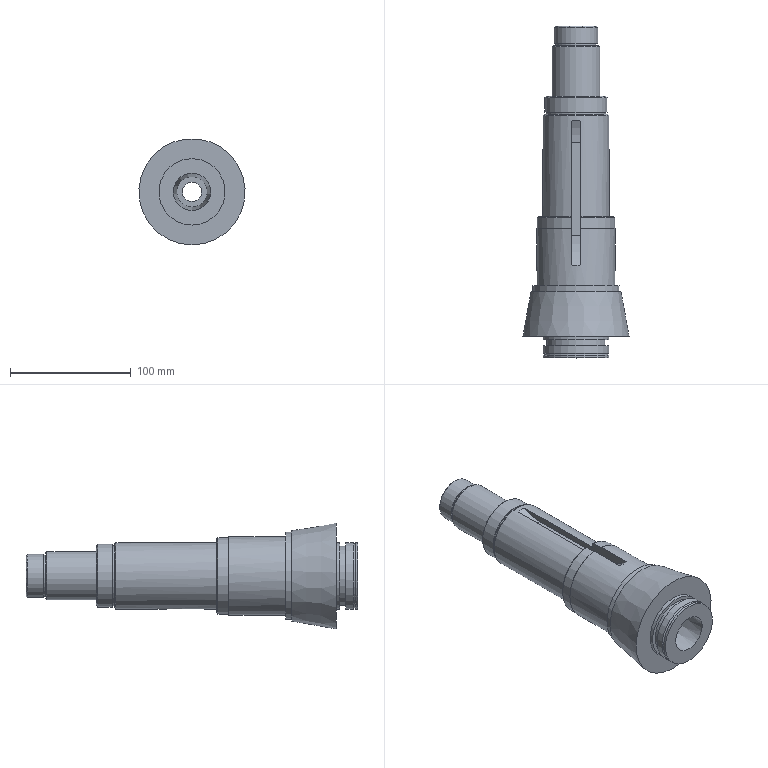Part | NX | features DATUM_CSYS 4, SKETCH 3, EXTRUDE 2, SYMBOLIC_THREAD 2, CHAMFER 1, DATUM_PLANE 1, SWP104 1 | 1 solid | 49 faces | box 88 x 275 x 88 mm | volume 636397 mm3 | plane 22 | cylinder 19 | cone 7 | torus 1 | commonest cylinder face diameters 55 x4 8 x2 70 x2 16 x1 28 x1 34 x1
STEP:
#1=CARTESIAN_POINT('',(0.,0.,-15.5));
#2=VERTEX_POINT('',#1);
#3=CARTESIAN_POINT('',(0.,0.,0.));
#4=DIRECTION('',(0.,-1.,0.));
#5=DIRECTION('',(0.,0.,-1.));
#6=AXIS2_PLACEMENT_3D('',#3,#4,#5);
#7=CIRCLE('',#6,15.5);
#8=EDGE_CURVE('',#2,#2,#7,.F.);
#9=ORIENTED_EDGE('',*,*,#8,.T.);
#10=EDGE_LOOP('',(#9));
#11=FACE_BOUND('',#10,.T.);
#12=CARTESIAN_POINT('',(0.,0.,-27.5));
#13=VERTEX_POINT('',#12);
#14=CARTESIAN_POINT('',(0.,0.,0.));
#15=DIRECTION('',(0.,-1.,0.));
#16=DIRECTION('',(0.,0.,-1.));
#17=AXIS2_PLACEMENT_3D('',#14,#15,#16);
#18=CIRCLE('',#17,27.5);
#19=EDGE_CURVE('',#13,#13,#18,.F.);
#20=ORIENTED_EDGE('',*,*,#19,.F.);
#21=EDGE_LOOP('',(#20));
#22=FACE_BOUND('',#21,.T.);
#23=CARTESIAN_POINT('',(0.,0.,27.5));
#24=DIRECTION('',(0.,1.,0.));
#25=DIRECTION('',(0.,0.,1.));
#26=AXIS2_PLACEMENT_3D('',#23,#24,#25);
#27=PLANE('',#26);
#28=ADVANCED_FACE('',(#11,#22),#27,.F.);
#29=CARTESIAN_POINT('',(0.,92.,-12.625));
#30=VERTEX_POINT('',#29);
#31=CARTESIAN_POINT('',(0.,92.,0.));
#32=DIRECTION('',(0.,-1.,0.));
#33=DIRECTION('',(0.,0.,-1.));
#34=AXIS2_PLACEMENT_3D('',#31,#32,#33);
#35=CIRCLE('',#34,12.625);
#36=EDGE_CURVE('',#30,#30,#35,.F.);
#37=ORIENTED_EDGE('',*,*,#36,.T.);
#38=EDGE_LOOP('',(#37));
#39=FACE_BOUND('',#38,.T.);
#40=ORIENTED_EDGE('',*,*,#8,.F.);
#41=EDGE_LOOP('',(#40));
#42=FACE_BOUND('',#41,.T.);
#43=CARTESIAN_POINT('',(0.,0.,0.));
#44=DIRECTION('',(0.,-1.,0.));
#45=DIRECTION('',(0.,0.,-1.));
#46=AXIS2_PLACEMENT_3D('',#43,#44,#45);
#47=CONICAL_SURFACE('',#46,15.5,0.03124);
#48=ADVANCED_FACE('',(#39,#42),#47,.F.);
#49=CARTESIAN_POINT('',(0.,92.,-14.));
#50=VERTEX_POINT('',#49);
#51=CARTESIAN_POINT('',(0.,92.,0.));
#52=DIRECTION('',(0.,-1.,0.));
#53=DIRECTION('',(0.,0.,-1.));
#54=AXIS2_PLACEMENT_3D('',#51,#52,#53);
#55=CIRCLE('',#54,14.);
#56=EDGE_CURVE('',#50,#50,#55,.F.);
#57=ORIENTED_EDGE('',*,*,#56,.T.);
#58=EDGE_LOOP('',(#57));
#59=FACE_BOUND('',#58,.T.);
#60=ORIENTED_EDGE('',*,*,#36,.F.);
#61=EDGE_LOOP('',(#60));
#62=FACE_BOUND('',#61,.T.);
#63=CARTESIAN_POINT('',(0.,92.,12.625));
#64=DIRECTION('',(0.,-1.,0.));
#65=DIRECTION('',(0.,0.,-1.));
#66=AXIS2_PLACEMENT_3D('',#63,#64,#65);
#67=PLANE('',#66);
#68=ADVANCED_FACE('',(#59,#62),#67,.F.);
#69=CARTESIAN_POINT('',(0.,107.,-14.));
#70=VERTEX_POINT('',#69);
#71=CARTESIAN_POINT('',(0.,107.,0.));
#72=DIRECTION('',(0.,-1.,0.));
#73=DIRECTION('',(0.,0.,-1.));
#74=AXIS2_PLACEMENT_3D('',#71,#72,#73);
#75=CIRCLE('',#74,14.);
#76=EDGE_CURVE('',#70,#70,#75,.F.);
#77=ORIENTED_EDGE('',*,*,#76,.T.);
#78=EDGE_LOOP('',(#77));
#79=FACE_BOUND('',#78,.T.);
#80=ORIENTED_EDGE('',*,*,#56,.F.);
#81=EDGE_LOOP('',(#80));
#82=FACE_BOUND('',#81,.T.);
#83=CARTESIAN_POINT('',(0.,0.,0.));
#84=DIRECTION('',(0.,-1.,0.));
#85=DIRECTION('',(0.,0.,-1.));
#86=AXIS2_PLACEMENT_3D('',#83,#84,#85);
#87=CYLINDRICAL_SURFACE('',#86,14.);
#88=ADVANCED_FACE('',(#79,#82),#87,.F.);
#89=CARTESIAN_POINT('',(0.,107.,-8.));
#90=VERTEX_POINT('',#89);
#91=CARTESIAN_POINT('',(0.,107.,0.));
#92=DIRECTION('',(0.,-1.,0.));
#93=DIRECTION('',(0.,0.,-1.));
#94=AXIS2_PLACEMENT_3D('',#91,#92,#93);
#95=CIRCLE('',#94,8.);
#96=EDGE_CURVE('',#90,#90,#95,.T.);
#97=ORIENTED_EDGE('',*,*,#96,.F.);
#98=EDGE_LOOP('',(#97));
#99=FACE_BOUND('',#98,.T.);
#100=ORIENTED_EDGE('',*,*,#76,.F.);
#101=EDGE_LOOP('',(#100));
#102=FACE_BOUND('',#101,.T.);
#103=CARTESIAN_POINT('',(0.,107.,14.));
#104=DIRECTION('',(0.,1.,0.));
#105=DIRECTION('',(0.,0.,1.));
#106=AXIS2_PLACEMENT_3D('',#103,#104,#105);
#107=PLANE('',#106);
#108=ADVANCED_FACE('',(#99,#102),#107,.F.);
#109=CARTESIAN_POINT('',(0.,275.,-8.));
#110=VERTEX_POINT('',#109);
#111=CARTESIAN_POINT('',(0.,275.,0.));
#112=DIRECTION('',(0.,-1.,0.));
#113=DIRECTION('',(0.,0.,-1.));
#114=AXIS2_PLACEMENT_3D('',#111,#112,#113);
#115=CIRCLE('',#114,8.);
#116=EDGE_CURVE('',#110,#110,#115,.T.);
#117=ORIENTED_EDGE('',*,*,#116,.F.);
#118=EDGE_LOOP('',(#117));
#119=FACE_BOUND('',#118,.T.);
#120=ORIENTED_EDGE('',*,*,#96,.T.);
#121=EDGE_LOOP('',(#120));
#122=FACE_BOUND('',#121,.T.);
#123=CARTESIAN_POINT('',(0.,0.,0.));
#124=DIRECTION('',(0.,-1.,0.));
#125=DIRECTION('',(0.,0.,-1.));
#126=AXIS2_PLACEMENT_3D('',#123,#124,#125);
#127=CYLINDRICAL_SURFACE('',#126,8.);
#128=ADVANCED_FACE('',(#119,#122),#127,.F.);
#129=CARTESIAN_POINT('',(0.,275.,-17.));
#130=VERTEX_POINT('',#129);
#131=CARTESIAN_POINT('',(0.,275.,0.));
#132=DIRECTION('',(0.,-1.,0.));
#133=DIRECTION('',(0.,0.,-1.));
#134=AXIS2_PLACEMENT_3D('',#131,#132,#133);
#135=CIRCLE('',#134,17.);
#136=EDGE_CURVE('',#130,#130,#135,.F.);
#137=ORIENTED_EDGE('',*,*,#136,.T.);
#138=EDGE_LOOP('',(#137));
#139=FACE_BOUND('',#138,.T.);
#140=ORIENTED_EDGE('',*,*,#116,.T.);
#141=EDGE_LOOP('',(#140));
#142=FACE_BOUND('',#141,.T.);
#143=CARTESIAN_POINT('',(0.,275.,8.));
#144=DIRECTION('',(0.,-1.,0.));
#145=DIRECTION('',(0.,0.,-1.));
#146=AXIS2_PLACEMENT_3D('',#143,#144,#145);
#147=PLANE('',#146);
#148=ADVANCED_FACE('',(#139,#142),#147,.F.);
#149=CARTESIAN_POINT('',(0.,274.,-18.));
#150=VERTEX_POINT('',#149);
#151=CARTESIAN_POINT('',(0.,274.,0.));
#152=DIRECTION('',(0.,-1.,0.));
#153=DIRECTION('',(0.,0.,-1.));
#154=AXIS2_PLACEMENT_3D('',#151,#152,#153);
#155=CIRCLE('',#154,18.);
#156=EDGE_CURVE('',#150,#150,#155,.T.);
#157=ORIENTED_EDGE('',*,*,#156,.T.);
#158=EDGE_LOOP('',(#157));
#159=FACE_BOUND('',#158,.T.);
#160=CARTESIAN_POINT('',(0.,260.7,-18.));
#161=VERTEX_POINT('',#160);
#162=CARTESIAN_POINT('',(0.,260.7,0.));
#163=DIRECTION('',(0.,-1.,0.));
#164=DIRECTION('',(0.,0.,-1.));
#165=AXIS2_PLACEMENT_3D('',#162,#163,#164);
#166=CIRCLE('',#165,18.);
#167=EDGE_CURVE('',#161,#161,#166,.F.);
#168=ORIENTED_EDGE('',*,*,#167,.T.);
#169=EDGE_LOOP('',(#168));
#170=FACE_BOUND('',#169,.T.);
#171=CARTESIAN_POINT('',(0.,0.,0.));
#172=DIRECTION('',(0.,-1.,0.));
#173=DIRECTION('',(0.,0.,-1.));
#174=AXIS2_PLACEMENT_3D('',#171,#172,#173);
#175=CYLINDRICAL_SURFACE('',#174,18.);
#176=ADVANCED_FACE('',(#159,#170),#175,.T.);
#177=CARTESIAN_POINT('',(0.,260.7,-17.));
#178=VERTEX_POINT('',#177);
#179=CARTESIAN_POINT('',(0.,260.7,0.));
#180=DIRECTION('',(0.,-1.,0.));
#181=DIRECTION('',(0.,0.,-1.));
#182=AXIS2_PLACEMENT_3D('',#179,#180,#181);
#183=CIRCLE('',#182,17.);
#184=EDGE_CURVE('',#178,#178,#183,.F.);
#185=ORIENTED_EDGE('',*,*,#184,.T.);
#186=EDGE_LOOP('',(#185));
#187=FACE_BOUND('',#186,.T.);
#188=ORIENTED_EDGE('',*,*,#167,.F.);
#189=EDGE_LOOP('',(#188));
#190=FACE_BOUND('',#189,.T.);
#191=CARTESIAN_POINT('',(0.,260.7,18.));
#192=DIRECTION('',(0.,1.,0.));
#193=DIRECTION('',(0.,0.,1.));
#194=AXIS2_PLACEMENT_3D('',#191,#192,#193);
#195=PLANE('',#194);
#196=ADVANCED_FACE('',(#187,#190),#195,.F.);
#197=CARTESIAN_POINT('',(0.,258.7,-17.));
#198=VERTEX_POINT('',#197);
#199=CARTESIAN_POINT('',(0.,258.7,0.));
#200=DIRECTION('',(0.,-1.,0.));
#201=DIRECTION('',(0.,0.,-1.));
#202=AXIS2_PLACEMENT_3D('',#199,#200,#201);
#203=CIRCLE('',#202,17.);
#204=EDGE_CURVE('',#198,#198,#203,.F.);
#205=ORIENTED_EDGE('',*,*,#204,.T.);
#206=EDGE_LOOP('',(#205));
#207=FACE_BOUND('',#206,.T.);
#208=ORIENTED_EDGE('',*,*,#184,.F.);
#209=EDGE_LOOP('',(#208));
#210=FACE_BOUND('',#209,.T.);
#211=CARTESIAN_POINT('',(0.,0.,0.));
#212=DIRECTION('',(0.,-1.,0.));
#213=DIRECTION('',(0.,0.,-1.));
#214=AXIS2_PLACEMENT_3D('',#211,#212,#213);
#215=CYLINDRICAL_SURFACE('',#214,17.);
#216=ADVANCED_FACE('',(#207,#210),#215,.T.);
#217=CARTESIAN_POINT('',(0.,258.7,-19.));
#218=VERTEX_POINT('',#217);
#219=CARTESIAN_POINT('',(0.,258.7,0.));
#220=DIRECTION('',(0.,-1.,0.));
#221=DIRECTION('',(0.,0.,-1.));
#222=AXIS2_PLACEMENT_3D('',#219,#220,#221);
#223=CIRCLE('',#222,19.);
#224=EDGE_CURVE('',#218,#218,#223,.F.);
#225=ORIENTED_EDGE('',*,*,#224,.T.);
#226=EDGE_LOOP('',(#225));
#227=FACE_BOUND('',#226,.T.);
#228=ORIENTED_EDGE('',*,*,#204,.F.);
#229=EDGE_LOOP('',(#228));
#230=FACE_BOUND('',#229,.T.);
#231=CARTESIAN_POINT('',(0.,258.7,17.));
#232=DIRECTION('',(0.,-1.,0.));
#233=DIRECTION('',(0.,0.,-1.));
#234=AXIS2_PLACEMENT_3D('',#231,#232,#233);
#235=PLANE('',#234);
#236=ADVANCED_FACE('',(#227,#230),#235,.F.);
#237=CARTESIAN_POINT('',(0.,257.7,-20.));
#238=VERTEX_POINT('',#237);
#239=CARTESIAN_POINT('',(0.,257.7,0.));
#240=DIRECTION('',(0.,-1.,0.));
#241=DIRECTION('',(0.,0.,-1.));
#242=AXIS2_PLACEMENT_3D('',#239,#240,#241);
#243=CIRCLE('',#242,20.);
#244=EDGE_CURVE('',#238,#238,#243,.T.);
#245=ORIENTED_EDGE('',*,*,#244,.T.);
#246=EDGE_LOOP('',(#245));
#247=FACE_BOUND('',#246,.T.);
#248=CARTESIAN_POINT('',(0.,216.7,-20.));
#249=VERTEX_POINT('',#248);
#250=CARTESIAN_POINT('',(0.,216.7,0.));
#251=DIRECTION('',(0.,-1.,0.));
#252=DIRECTION('',(0.,0.,-1.));
#253=AXIS2_PLACEMENT_3D('',#250,#251,#252);
#254=CIRCLE('',#253,20.);
#255=EDGE_CURVE('',#249,#249,#254,.F.);
#256=ORIENTED_EDGE('',*,*,#255,.T.);
#257=EDGE_LOOP('',(#256));
#258=FACE_BOUND('',#257,.T.);
#259=CARTESIAN_POINT('',(0.,0.,0.));
#260=DIRECTION('',(0.,-1.,0.));
#261=DIRECTION('',(0.,0.,-1.));
#262=AXIS2_PLACEMENT_3D('',#259,#260,#261);
#263=CYLINDRICAL_SURFACE('',#262,20.);
#264=ADVANCED_FACE('',(#247,#258),#263,.T.);
#265=CARTESIAN_POINT('',(0.,216.7,-25.));
#266=VERTEX_POINT('',#265);
#267=CARTESIAN_POINT('',(0.,216.7,0.));
#268=DIRECTION('',(0.,-1.,0.));
#269=DIRECTION('',(0.,0.,-1.));
#270=AXIS2_PLACEMENT_3D('',#267,#268,#269);
#271=CIRCLE('',#270,25.);
#272=EDGE_CURVE('',#266,#266,#271,.F.);
#273=ORIENTED_EDGE('',*,*,#272,.T.);
#274=EDGE_LOOP('',(#273));
#275=FACE_BOUND('',#274,.T.);
#276=ORIENTED_EDGE('',*,*,#255,.F.);
#277=EDGE_LOOP('',(#276));
#278=FACE_BOUND('',#277,.T.);
#279=CARTESIAN_POINT('',(0.,216.7,20.));
#280=DIRECTION('',(0.,-1.,0.));
#281=DIRECTION('',(0.,0.,-1.));
#282=AXIS2_PLACEMENT_3D('',#279,#280,#281);
#283=PLANE('',#282);
#284=ADVANCED_FACE('',(#275,#278),#283,.F.);
#285=CARTESIAN_POINT('',(0.,215.7,-26.));
#286=VERTEX_POINT('',#285);
#287=CARTESIAN_POINT('',(0.,215.7,0.));
#288=DIRECTION('',(0.,-1.,0.));
#289=DIRECTION('',(0.,0.,-1.));
#290=AXIS2_PLACEMENT_3D('',#287,#288,#289);
#291=CIRCLE('',#290,26.);
#292=EDGE_CURVE('',#286,#286,#291,.T.);
#293=ORIENTED_EDGE('',*,*,#292,.T.);
#294=EDGE_LOOP('',(#293));
#295=FACE_BOUND('',#294,.T.);
#296=CARTESIAN_POINT('',(0.,203.7,-26.));
#297=VERTEX_POINT('',#296);
#298=CARTESIAN_POINT('',(0.,203.7,0.));
#299=DIRECTION('',(0.,-1.,0.));
#300=DIRECTION('',(0.,0.,-1.));
#301=AXIS2_PLACEMENT_3D('',#298,#299,#300);
#302=CIRCLE('',#301,26.);
#303=EDGE_CURVE('',#297,#297,#302,.F.);
#304=ORIENTED_EDGE('',*,*,#303,.T.);
#305=EDGE_LOOP('',(#304));
#306=FACE_BOUND('',#305,.T.);
#307=CARTESIAN_POINT('',(0.,0.,0.));
#308=DIRECTION('',(0.,-1.,0.));
#309=DIRECTION('',(0.,0.,-1.));
#310=AXIS2_PLACEMENT_3D('',#307,#308,#309);
#311=CYLINDRICAL_SURFACE('',#310,26.);
#312=ADVANCED_FACE('',(#295,#306),#311,.T.);
#313=CARTESIAN_POINT('',(0.,203.7,-25.));
#314=VERTEX_POINT('',#313);
#315=CARTESIAN_POINT('',(0.,203.7,0.));
#316=DIRECTION('',(0.,-1.,0.));
#317=DIRECTION('',(0.,0.,-1.));
#318=AXIS2_PLACEMENT_3D('',#315,#316,#317);
#319=CIRCLE('',#318,25.);
#320=EDGE_CURVE('',#314,#314,#319,.F.);
#321=ORIENTED_EDGE('',*,*,#320,.T.);
#322=EDGE_LOOP('',(#321));
#323=FACE_BOUND('',#322,.T.);
#324=ORIENTED_EDGE('',*,*,#303,.F.);
#325=EDGE_LOOP('',(#324));
#326=FACE_BOUND('',#325,.T.);
#327=CARTESIAN_POINT('',(0.,203.7,26.));
#328=DIRECTION('',(0.,1.,0.));
#329=DIRECTION('',(0.,0.,1.));
#330=AXIS2_PLACEMENT_3D('',#327,#328,#329);
#331=PLANE('',#330);
#332=ADVANCED_FACE('',(#323,#326),#331,.F.);
#333=CARTESIAN_POINT('',(0.,201.7,-25.));
#334=VERTEX_POINT('',#333);
#335=CARTESIAN_POINT('',(0.,201.7,0.));
#336=DIRECTION('',(0.,-1.,0.));
#337=DIRECTION('',(0.,0.,-1.));
#338=AXIS2_PLACEMENT_3D('',#335,#336,#337);
#339=CIRCLE('',#338,25.);
#340=EDGE_CURVE('',#334,#334,#339,.F.);
#341=ORIENTED_EDGE('',*,*,#340,.T.);
#342=EDGE_LOOP('',(#341));
#343=FACE_BOUND('',#342,.T.);
#344=ORIENTED_EDGE('',*,*,#320,.F.);
#345=EDGE_LOOP('',(#344));
#346=FACE_BOUND('',#345,.T.);
#347=CARTESIAN_POINT('',(0.,0.,0.));
#348=DIRECTION('',(0.,-1.,0.));
#349=DIRECTION('',(0.,0.,-1.));
#350=AXIS2_PLACEMENT_3D('',#347,#348,#349);
#351=CYLINDRICAL_SURFACE('',#350,25.);
#352=ADVANCED_FACE('',(#343,#346),#351,.T.);
#353=CARTESIAN_POINT('',(0.,201.7,-26.5));
#354=VERTEX_POINT('',#353);
#355=CARTESIAN_POINT('',(0.,201.7,0.));
#356=DIRECTION('',(0.,-1.,0.));
#357=DIRECTION('',(0.,0.,-1.));
#358=AXIS2_PLACEMENT_3D('',#355,#356,#357);
#359=CIRCLE('',#358,26.5);
#360=EDGE_CURVE('',#354,#354,#359,.F.);
#361=ORIENTED_EDGE('',*,*,#360,.T.);
#362=EDGE_LOOP('',(#361));
#363=FACE_BOUND('',#362,.T.);
#364=ORIENTED_EDGE('',*,*,#340,.F.);
#365=EDGE_LOOP('',(#364));
#366=FACE_BOUND('',#365,.T.);
#367=CARTESIAN_POINT('',(0.,201.7,25.));
#368=DIRECTION('',(0.,-1.,0.));
#369=DIRECTION('',(0.,0.,-1.));
#370=AXIS2_PLACEMENT_3D('',#367,#368,#369);
#371=PLANE('',#370);
#372=ADVANCED_FACE('',(#363,#366),#371,.F.);
#373=CARTESIAN_POINT('',(0.,200.7,-27.5));
#374=VERTEX_POINT('',#373);
#375=CARTESIAN_POINT('',(0.,200.7,0.));
#376=DIRECTION('',(0.,-1.,0.));
#377=DIRECTION('',(0.,0.,-1.));
#378=AXIS2_PLACEMENT_3D('',#375,#376,#377);
#379=CIRCLE('',#378,27.5);
#380=EDGE_CURVE('',#374,#374,#379,.T.);
#381=ORIENTED_EDGE('',*,*,#380,.T.);
#382=EDGE_LOOP('',(#381));
#383=FACE_BOUND('',#382,.T.);
#384=CARTESIAN_POINT('',(-4.,131.,-27.208));
#385=VERTEX_POINT('',#384);
#386=CARTESIAN_POINT('',(-4.,155.,-27.208));
#387=VERTEX_POINT('',#386);
#388=CARTESIAN_POINT('',(-4.,0.,-27.208));
#389=DIRECTION('',(0.,-1.,0.));
#390=VECTOR('',#389,1000.);
#391=LINE('',#388,#390);
#392=EDGE_CURVE('',#385,#387,#391,.F.);
#393=ORIENTED_EDGE('',*,*,#392,.F.);
#394=CARTESIAN_POINT('',(4.,131.,-27.208));
#395=VERTEX_POINT('',#394);
#396=CARTESIAN_POINT('',(-4.,131.,-27.208));
#397=CARTESIAN_POINT('',(-4.,129.942,-27.208));
#398=CARTESIAN_POINT('',(-3.133,127.872,-27.355));
#399=CARTESIAN_POINT('',(-0.004382,126.565,-27.573));
#400=CARTESIAN_POINT('',(3.133,127.869,-27.355));
#401=CARTESIAN_POINT('',(4.,129.942,-27.208));
#402=CARTESIAN_POINT('',(4.,131.,-27.208));
#403=B_SPLINE_CURVE_WITH_KNOTS('',3,(#396,#397,#398,#399,#400,#401,#402),.UNSPECIFIED.,.F.,.F.,(4,1,1,1,4),(0.,0.00313,0.00626,0.00939,0.01252),.UNSPECIFIED.);
#404=EDGE_CURVE('',#395,#385,#403,.F.);
#405=ORIENTED_EDGE('',*,*,#404,.F.);
#406=CARTESIAN_POINT('',(4.,155.,-27.208));
#407=VERTEX_POINT('',#406);
#408=CARTESIAN_POINT('',(4.,0.,-27.208));
#409=DIRECTION('',(0.,-1.,0.));
#410=VECTOR('',#409,1000.);
#411=LINE('',#408,#410);
#412=EDGE_CURVE('',#407,#395,#411,.T.);
#413=ORIENTED_EDGE('',*,*,#412,.F.);
#414=CARTESIAN_POINT('',(4.,155.,-27.208));
#415=CARTESIAN_POINT('',(4.,156.058,-27.208));
#416=CARTESIAN_POINT('',(3.133,158.128,-27.355));
#417=CARTESIAN_POINT('',(0.004382,159.435,-27.573));
#418=CARTESIAN_POINT('',(-3.133,158.131,-27.355));
#419=CARTESIAN_POINT('',(-4.,156.058,-27.208));
#420=CARTESIAN_POINT('',(-4.,155.,-27.208));
#421=B_SPLINE_CURVE_WITH_KNOTS('',3,(#414,#415,#416,#417,#418,#419,#420),.UNSPECIFIED.,.F.,.F.,(4,1,1,1,4),(0.,0.00313,0.00626,0.00939,0.01252),.UNSPECIFIED.);
#422=EDGE_CURVE('',#387,#407,#421,.F.);
#423=ORIENTED_EDGE('',*,*,#422,.F.);
#424=EDGE_LOOP('',(#393,#405,#413,#423));
#425=FACE_BOUND('',#424,.T.);
#426=CARTESIAN_POINT('',(-4.,196.204,27.208));
#427=VERTEX_POINT('',#426);
#428=CARTESIAN_POINT('',(4.,196.204,27.208));
#429=VERTEX_POINT('',#428);
#430=CARTESIAN_POINT('',(4.,196.204,27.208));
#431=CARTESIAN_POINT('',(1.387,196.868,27.592));
#432=CARTESIAN_POINT('',(-1.387,196.868,27.592));
#433=CARTESIAN_POINT('',(-4.,196.204,27.208));
#434=B_SPLINE_CURVE_WITH_KNOTS('',3,(#430,#431,#432,#433),.UNSPECIFIED.,.F.,.F.,(4,4),(0.,0.008055),.UNSPECIFIED.);
#435=EDGE_CURVE('',#427,#429,#434,.F.);
#436=ORIENTED_EDGE('',*,*,#435,.T.);
#437=CARTESIAN_POINT('',(4.,117.,27.208));
#438=VERTEX_POINT('',#437);
#439=CARTESIAN_POINT('',(4.,0.,27.208));
#440=DIRECTION('',(0.,-1.,0.));
#441=VECTOR('',#440,1000.);
#442=LINE('',#439,#441);
#443=EDGE_CURVE('',#438,#429,#442,.F.);
#444=ORIENTED_EDGE('',*,*,#443,.F.);
#445=CARTESIAN_POINT('',(-4.,117.,27.208));
#446=VERTEX_POINT('',#445);
#447=CARTESIAN_POINT('',(0.,117.,0.));
#448=DIRECTION('',(0.,-1.,0.));
#449=DIRECTION('',(0.,0.,-1.));
#450=AXIS2_PLACEMENT_3D('',#447,#448,#449);
#451=CIRCLE('',#450,27.5);
#452=EDGE_CURVE('',#438,#446,#451,.F.);
#453=ORIENTED_EDGE('',*,*,#452,.T.);
#454=CARTESIAN_POINT('',(-4.,0.,27.208));
#455=DIRECTION('',(0.,-1.,0.));
#456=VECTOR('',#455,1000.);
#457=LINE('',#454,#456);
#458=EDGE_CURVE('',#446,#427,#457,.F.);
#459=ORIENTED_EDGE('',*,*,#458,.T.);
#460=EDGE_LOOP('',(#436,#444,#453,#459));
#461=FACE_BOUND('',#460,.T.);
#462=CARTESIAN_POINT('',(0.,0.,0.));
#463=DIRECTION('',(0.,-1.,0.));
#464=DIRECTION('',(0.,0.,-1.));
#465=AXIS2_PLACEMENT_3D('',#462,#463,#464);
#466=CYLINDRICAL_SURFACE('',#465,27.5);
#467=ADVANCED_FACE('',(#383,#425,#461),#466,.T.);
#468=CARTESIAN_POINT('',(4.,117.,30.741));
#469=VERTEX_POINT('',#468);
#470=CARTESIAN_POINT('',(4.,117.,27.5));
#471=DIRECTION('',(0.,0.,1.));
#472=VECTOR('',#471,1000.);
#473=LINE('',#470,#472);
#474=EDGE_CURVE('',#469,#438,#473,.F.);
#475=ORIENTED_EDGE('',*,*,#474,.F.);
#476=CARTESIAN_POINT('',(-4.,117.,30.741));
#477=VERTEX_POINT('',#476);
#478=CARTESIAN_POINT('',(0.,117.,0.));
#479=DIRECTION('',(0.,-1.,0.));
#480=DIRECTION('',(0.,0.,-1.));
#481=AXIS2_PLACEMENT_3D('',#478,#479,#480);
#482=CIRCLE('',#481,31.);
#483=EDGE_CURVE('',#469,#477,#482,.F.);
#484=ORIENTED_EDGE('',*,*,#483,.T.);
#485=CARTESIAN_POINT('',(-4.,117.,27.5));
#486=DIRECTION('',(0.,0.,1.));
#487=VECTOR('',#486,1000.);
#488=LINE('',#485,#487);
#489=EDGE_CURVE('',#477,#446,#488,.F.);
#490=ORIENTED_EDGE('',*,*,#489,.T.);
#491=ORIENTED_EDGE('',*,*,#452,.F.);
#492=EDGE_LOOP('',(#475,#484,#490,#491));
#493=FACE_BOUND('',#492,.T.);
#494=CARTESIAN_POINT('',(0.,117.,27.5));
#495=DIRECTION('',(0.,-1.,0.));
#496=DIRECTION('',(0.,0.,-1.));
#497=AXIS2_PLACEMENT_3D('',#494,#495,#496);
#498=PLANE('',#497);
#499=ADVANCED_FACE('',(#493),#498,.F.);
#500=CARTESIAN_POINT('',(-4.,107.,31.749));
#501=VERTEX_POINT('',#500);
#502=CARTESIAN_POINT('',(-4.,116.,31.749));
#503=VERTEX_POINT('',#502);
#504=CARTESIAN_POINT('',(-4.,0.,31.749));
#505=DIRECTION('',(0.,-1.,0.));
#506=VECTOR('',#505,1000.);
#507=LINE('',#504,#506);
#508=EDGE_CURVE('',#501,#503,#507,.F.);
#509=ORIENTED_EDGE('',*,*,#508,.T.);
#510=CARTESIAN_POINT('',(4.,116.,31.749));
#511=VERTEX_POINT('',#510);
#512=CARTESIAN_POINT('',(0.,116.,0.));
#513=DIRECTION('',(0.,-1.,0.));
#514=DIRECTION('',(0.,0.,-1.));
#515=AXIS2_PLACEMENT_3D('',#512,#513,#514);
#516=CIRCLE('',#515,32.);
#517=EDGE_CURVE('',#503,#511,#516,.T.);
#518=ORIENTED_EDGE('',*,*,#517,.T.);
#519=CARTESIAN_POINT('',(4.,107.,31.749));
#520=VERTEX_POINT('',#519);
#521=CARTESIAN_POINT('',(4.,0.,31.749));
#522=DIRECTION('',(0.,-1.,0.));
#523=VECTOR('',#522,1000.);
#524=LINE('',#521,#523);
#525=EDGE_CURVE('',#520,#511,#524,.F.);
#526=ORIENTED_EDGE('',*,*,#525,.F.);
#527=CARTESIAN_POINT('',(0.,107.,0.));
#528=DIRECTION('',(0.,-1.,0.));
#529=DIRECTION('',(0.,0.,-1.));
#530=AXIS2_PLACEMENT_3D('',#527,#528,#529);
#531=CIRCLE('',#530,32.);
#532=EDGE_CURVE('',#520,#501,#531,.F.);
#533=ORIENTED_EDGE('',*,*,#532,.T.);
#534=EDGE_LOOP('',(#509,#518,#526,#533));
#535=FACE_BOUND('',#534,.T.);
#536=CARTESIAN_POINT('',(0.,0.,0.));
#537=DIRECTION('',(0.,-1.,0.));
#538=DIRECTION('',(0.,0.,-1.));
#539=AXIS2_PLACEMENT_3D('',#536,#537,#538);
#540=CYLINDRICAL_SURFACE('',#539,32.);
#541=ADVANCED_FACE('',(#535),#540,.T.);
#542=ORIENTED_EDGE('',*,*,#532,.F.);
#543=CARTESIAN_POINT('',(4.,107.,32.253));
#544=VERTEX_POINT('',#543);
#545=CARTESIAN_POINT('',(4.,107.,32.));
#546=DIRECTION('',(0.,0.,1.));
#547=VECTOR('',#546,1000.);
#548=LINE('',#545,#547);
#549=EDGE_CURVE('',#544,#520,#548,.F.);
#550=ORIENTED_EDGE('',*,*,#549,.F.);
#551=CARTESIAN_POINT('',(-4.,107.,32.253));
#552=VERTEX_POINT('',#551);
#553=CARTESIAN_POINT('',(0.,107.,0.));
#554=DIRECTION('',(0.,-1.,0.));
#555=DIRECTION('',(0.,0.,-1.));
#556=AXIS2_PLACEMENT_3D('',#553,#554,#555);
#557=CIRCLE('',#556,32.5);
#558=EDGE_CURVE('',#544,#552,#557,.F.);
#559=ORIENTED_EDGE('',*,*,#558,.T.);
#560=CARTESIAN_POINT('',(-4.,107.,32.));
#561=DIRECTION('',(0.,0.,1.));
#562=VECTOR('',#561,1000.);
#563=LINE('',#560,#562);
#564=EDGE_CURVE('',#552,#501,#563,.F.);
#565=ORIENTED_EDGE('',*,*,#564,.T.);
#566=EDGE_LOOP('',(#542,#550,#559,#565));
#567=FACE_BOUND('',#566,.T.);
#568=CARTESIAN_POINT('',(0.,107.,32.));
#569=DIRECTION('',(0.,-1.,0.));
#570=DIRECTION('',(0.,0.,-1.));
#571=AXIS2_PLACEMENT_3D('',#568,#569,#570);
#572=PLANE('',#571);
#573=ADVANCED_FACE('',(#567),#572,.F.);
#574=CARTESIAN_POINT('',(0.,60.,-32.5));
#575=VERTEX_POINT('',#574);
#576=CARTESIAN_POINT('',(0.,60.,0.));
#577=DIRECTION('',(0.,-1.,0.));
#578=DIRECTION('',(0.,0.,-1.));
#579=AXIS2_PLACEMENT_3D('',#576,#577,#578);
#580=CIRCLE('',#579,32.5);
#581=EDGE_CURVE('',#575,#575,#580,.F.);
#582=ORIENTED_EDGE('',*,*,#581,.T.);
#583=EDGE_LOOP('',(#582));
#584=FACE_BOUND('',#583,.T.);
#585=ORIENTED_EDGE('',*,*,#558,.F.);
#586=CARTESIAN_POINT('',(4.,76.955,32.253));
#587=VERTEX_POINT('',#586);
#588=CARTESIAN_POINT('',(4.,0.,32.253));
#589=DIRECTION('',(0.,-1.,0.));
#590=VECTOR('',#589,1000.);
#591=LINE('',#588,#590);
#592=EDGE_CURVE('',#587,#544,#591,.F.);
#593=ORIENTED_EDGE('',*,*,#592,.F.);
#594=CARTESIAN_POINT('',(-4.,76.955,32.253));
#595=VERTEX_POINT('',#594);
#596=CARTESIAN_POINT('',(-4.,76.955,32.253));
#597=CARTESIAN_POINT('',(-1.333,76.61,32.584));
#598=CARTESIAN_POINT('',(1.333,76.61,32.584));
#599=CARTESIAN_POINT('',(4.,76.955,32.253));
#600=B_SPLINE_CURVE_WITH_KNOTS('',3,(#596,#597,#598,#599),.UNSPECIFIED.,.F.,.F.,(4,4),(0.,0.008),.UNSPECIFIED.);
#601=EDGE_CURVE('',#587,#595,#600,.F.);
#602=ORIENTED_EDGE('',*,*,#601,.T.);
#603=CARTESIAN_POINT('',(-4.,0.,32.253));
#604=DIRECTION('',(0.,-1.,0.));
#605=VECTOR('',#604,1000.);
#606=LINE('',#603,#605);
#607=EDGE_CURVE('',#595,#552,#606,.F.);
#608=ORIENTED_EDGE('',*,*,#607,.T.);
#609=EDGE_LOOP('',(#585,#593,#602,#608));
#610=FACE_BOUND('',#609,.T.);
#611=CARTESIAN_POINT('',(0.,0.,0.));
#612=DIRECTION('',(0.,-1.,0.));
#613=DIRECTION('',(0.,0.,-1.));
#614=AXIS2_PLACEMENT_3D('',#611,#612,#613);
#615=CYLINDRICAL_SURFACE('',#614,32.5);
#616=ADVANCED_FACE('',(#584,#610),#615,.T.);
#617=CARTESIAN_POINT('',(0.,60.,-36.));
#618=VERTEX_POINT('',#617);
#619=CARTESIAN_POINT('',(0.,60.,0.));
#620=DIRECTION('',(0.,-1.,0.));
#621=DIRECTION('',(0.,0.,-1.));
#622=AXIS2_PLACEMENT_3D('',#619,#620,#621);
#623=CIRCLE('',#622,36.);
#624=EDGE_CURVE('',#618,#618,#623,.F.);
#625=ORIENTED_EDGE('',*,*,#624,.T.);
#626=EDGE_LOOP('',(#625));
#627=FACE_BOUND('',#626,.T.);
#628=ORIENTED_EDGE('',*,*,#581,.F.);
#629=EDGE_LOOP('',(#628));
#630=FACE_BOUND('',#629,.T.);
#631=CARTESIAN_POINT('',(0.,60.,32.5));
#632=DIRECTION('',(0.,-1.,0.));
#633=DIRECTION('',(0.,0.,-1.));
#634=AXIS2_PLACEMENT_3D('',#631,#632,#633);
#635=PLANE('',#634);
#636=ADVANCED_FACE('',(#627,#630),#635,.F.);
#637=CARTESIAN_POINT('',(0.,55.,-36.));
#638=VERTEX_POINT('',#637);
#639=CARTESIAN_POINT('',(0.,55.,0.));
#640=DIRECTION('',(0.,-1.,0.));
#641=DIRECTION('',(0.,0.,-1.));
#642=AXIS2_PLACEMENT_3D('',#639,#640,#641);
#643=CIRCLE('',#642,36.);
#644=EDGE_CURVE('',#638,#638,#643,.F.);
#645=ORIENTED_EDGE('',*,*,#644,.T.);
#646=EDGE_LOOP('',(#645));
#647=FACE_BOUND('',#646,.T.);
#648=ORIENTED_EDGE('',*,*,#624,.F.);
#649=EDGE_LOOP('',(#648));
#650=FACE_BOUND('',#649,.T.);
#651=CARTESIAN_POINT('',(0.,0.,0.));
#652=DIRECTION('',(0.,-1.,0.));
#653=DIRECTION('',(0.,0.,-1.));
#654=AXIS2_PLACEMENT_3D('',#651,#652,#653);
#655=CYLINDRICAL_SURFACE('',#654,36.);
#656=ADVANCED_FACE('',(#647,#650),#655,.T.);
#657=CARTESIAN_POINT('',(0.,55.,-37.476));
#658=VERTEX_POINT('',#657);
#659=CARTESIAN_POINT('',(0.,55.,0.));
#660=DIRECTION('',(0.,-1.,0.));
#661=DIRECTION('',(0.,0.,-1.));
#662=AXIS2_PLACEMENT_3D('',#659,#660,#661);
#663=CIRCLE('',#662,37.476);
#664=EDGE_CURVE('',#658,#658,#663,.F.);
#665=ORIENTED_EDGE('',*,*,#664,.T.);
#666=EDGE_LOOP('',(#665));
#667=FACE_BOUND('',#666,.T.);
#668=ORIENTED_EDGE('',*,*,#644,.F.);
#669=EDGE_LOOP('',(#668));
#670=FACE_BOUND('',#669,.T.);
#671=CARTESIAN_POINT('',(0.,55.,36.));
#672=DIRECTION('',(0.,-1.,0.));
#673=DIRECTION('',(0.,0.,-1.));
#674=AXIS2_PLACEMENT_3D('',#671,#672,#673);
#675=PLANE('',#674);
#676=ADVANCED_FACE('',(#667,#670),#675,.F.);
#677=CARTESIAN_POINT('',(0.,18.,-44.));
#678=VERTEX_POINT('',#677);
#679=CARTESIAN_POINT('',(0.,18.,0.));
#680=DIRECTION('',(0.,-1.,0.));
#681=DIRECTION('',(0.,0.,-1.));
#682=AXIS2_PLACEMENT_3D('',#679,#680,#681);
#683=CIRCLE('',#682,44.);
#684=EDGE_CURVE('',#678,#678,#683,.F.);
#685=ORIENTED_EDGE('',*,*,#684,.T.);
#686=EDGE_LOOP('',(#685));
#687=FACE_BOUND('',#686,.T.);
#688=ORIENTED_EDGE('',*,*,#664,.F.);
#689=EDGE_LOOP('',(#688));
#690=FACE_BOUND('',#689,.T.);
#691=CARTESIAN_POINT('',(0.,55.,0.));
#692=DIRECTION('',(0.,-1.,0.));
#693=DIRECTION('',(0.,0.,-1.));
#694=AXIS2_PLACEMENT_3D('',#691,#692,#693);
#695=CONICAL_SURFACE('',#694,37.476,0.1745);
#696=ADVANCED_FACE('',(#687,#690),#695,.T.);
#697=CARTESIAN_POINT('',(0.,18.,-27.5));
#698=VERTEX_POINT('',#697);
#699=CARTESIAN_POINT('',(0.,18.,0.));
#700=DIRECTION('',(0.,-1.,0.));
#701=DIRECTION('',(0.,0.,-1.));
#702=AXIS2_PLACEMENT_3D('',#699,#700,#701);
#703=CIRCLE('',#702,27.5);
#704=EDGE_CURVE('',#698,#698,#703,.F.);
#705=ORIENTED_EDGE('',*,*,#704,.T.);
#706=EDGE_LOOP('',(#705));
#707=FACE_BOUND('',#706,.T.);
#708=ORIENTED_EDGE('',*,*,#684,.F.);
#709=EDGE_LOOP('',(#708));
#710=FACE_BOUND('',#709,.T.);
#711=CARTESIAN_POINT('',(0.,18.,44.));
#712=DIRECTION('',(0.,1.,0.));
#713=DIRECTION('',(0.,0.,1.));
#714=AXIS2_PLACEMENT_3D('',#711,#712,#713);
#715=PLANE('',#714);
#716=ADVANCED_FACE('',(#707,#710),#715,.F.);
#717=CARTESIAN_POINT('',(0.,15.,-27.5));
#718=VERTEX_POINT('',#717);
#719=CARTESIAN_POINT('',(0.,15.,0.));
#720=DIRECTION('',(0.,-1.,0.));
#721=DIRECTION('',(0.,0.,-1.));
#722=AXIS2_PLACEMENT_3D('',#719,#720,#721);
#723=CIRCLE('',#722,27.5);
#724=EDGE_CURVE('',#718,#718,#723,.F.);
#725=ORIENTED_EDGE('',*,*,#724,.T.);
#726=EDGE_LOOP('',(#725));
#727=FACE_BOUND('',#726,.T.);
#728=ORIENTED_EDGE('',*,*,#704,.F.);
#729=EDGE_LOOP('',(#728));
#730=FACE_BOUND('',#729,.T.);
#731=CARTESIAN_POINT('',(0.,0.,0.));
#732=DIRECTION('',(0.,-1.,0.));
#733=DIRECTION('',(0.,0.,-1.));
#734=AXIS2_PLACEMENT_3D('',#731,#732,#733);
#735=CYLINDRICAL_SURFACE('',#734,27.5);
#736=ADVANCED_FACE('',(#727,#730),#735,.T.);
#737=CARTESIAN_POINT('',(0.,15.,-24.5));
#738=VERTEX_POINT('',#737);
#739=CARTESIAN_POINT('',(0.,15.,0.));
#740=DIRECTION('',(0.,-1.,0.));
#741=DIRECTION('',(0.,0.,-1.));
#742=AXIS2_PLACEMENT_3D('',#739,#740,#741);
#743=CIRCLE('',#742,24.5);
#744=EDGE_CURVE('',#738,#738,#743,.F.);
#745=ORIENTED_EDGE('',*,*,#744,.T.);
#746=EDGE_LOOP('',(#745));
#747=FACE_BOUND('',#746,.T.);
#748=ORIENTED_EDGE('',*,*,#724,.F.);
#749=EDGE_LOOP('',(#748));
#750=FACE_BOUND('',#749,.T.);
#751=CARTESIAN_POINT('',(0.,15.,27.5));
#752=DIRECTION('',(0.,1.,0.));
#753=DIRECTION('',(0.,0.,1.));
#754=AXIS2_PLACEMENT_3D('',#751,#752,#753);
#755=PLANE('',#754);
#756=ADVANCED_FACE('',(#747,#750),#755,.F.);
#757=CARTESIAN_POINT('',(0.,10.,-24.5));
#758=VERTEX_POINT('',#757);
#759=CARTESIAN_POINT('',(0.,10.,0.));
#760=DIRECTION('',(0.,-1.,0.));
#761=DIRECTION('',(0.,0.,-1.));
#762=AXIS2_PLACEMENT_3D('',#759,#760,#761);
#763=CIRCLE('',#762,24.5);
#764=EDGE_CURVE('',#758,#758,#763,.F.);
#765=ORIENTED_EDGE('',*,*,#764,.T.);
#766=EDGE_LOOP('',(#765));
#767=FACE_BOUND('',#766,.T.);
#768=ORIENTED_EDGE('',*,*,#744,.F.);
#769=EDGE_LOOP('',(#768));
#770=FACE_BOUND('',#769,.T.);
#771=CARTESIAN_POINT('',(0.,0.,0.));
#772=DIRECTION('',(0.,-1.,0.));
#773=DIRECTION('',(0.,0.,-1.));
#774=AXIS2_PLACEMENT_3D('',#771,#772,#773);
#775=CYLINDRICAL_SURFACE('',#774,24.5);
#776=ADVANCED_FACE('',(#767,#770),#775,.T.);
#777=CARTESIAN_POINT('',(0.,10.,-27.5));
#778=VERTEX_POINT('',#777);
#779=CARTESIAN_POINT('',(0.,10.,0.));
#780=DIRECTION('',(0.,-1.,0.));
#781=DIRECTION('',(0.,0.,-1.));
#782=AXIS2_PLACEMENT_3D('',#779,#780,#781);
#783=CIRCLE('',#782,27.5);
#784=EDGE_CURVE('',#778,#778,#783,.F.);
#785=ORIENTED_EDGE('',*,*,#784,.T.);
#786=EDGE_LOOP('',(#785));
#787=FACE_BOUND('',#786,.T.);
#788=ORIENTED_EDGE('',*,*,#764,.F.);
#789=EDGE_LOOP('',(#788));
#790=FACE_BOUND('',#789,.T.);
#791=CARTESIAN_POINT('',(0.,10.,24.5));
#792=DIRECTION('',(0.,-1.,0.));
#793=DIRECTION('',(0.,0.,-1.));
#794=AXIS2_PLACEMENT_3D('',#791,#792,#793);
#795=PLANE('',#794);
#796=ADVANCED_FACE('',(#787,#790),#795,.F.);
#797=CARTESIAN_POINT('',(0.,4.,-27.5));
#798=VERTEX_POINT('',#797);
#799=CARTESIAN_POINT('',(0.,4.,0.));
#800=DIRECTION('',(0.,-1.,0.));
#801=DIRECTION('',(0.,0.,-1.));
#802=AXIS2_PLACEMENT_3D('',#799,#800,#801);
#803=CIRCLE('',#802,27.5);
#804=EDGE_CURVE('',#798,#798,#803,.F.);
#805=ORIENTED_EDGE('',*,*,#804,.T.);
#806=EDGE_LOOP('',(#805));
#807=FACE_BOUND('',#806,.T.);
#808=ORIENTED_EDGE('',*,*,#784,.F.);
#809=EDGE_LOOP('',(#808));
#810=FACE_BOUND('',#809,.T.);
#811=CARTESIAN_POINT('',(0.,0.,0.));
#812=DIRECTION('',(0.,-1.,0.));
#813=DIRECTION('',(0.,0.,-1.));
#814=AXIS2_PLACEMENT_3D('',#811,#812,#813);
#815=CYLINDRICAL_SURFACE('',#814,27.5);
#816=ADVANCED_FACE('',(#807,#810),#815,.T.);
#817=CARTESIAN_POINT('',(0.,2.,-27.5));
#818=VERTEX_POINT('',#817);
#819=CARTESIAN_POINT('',(0.,2.,0.));
#820=DIRECTION('',(0.,-1.,0.));
#821=DIRECTION('',(0.,0.,-1.));
#822=AXIS2_PLACEMENT_3D('',#819,#820,#821);
#823=CIRCLE('',#822,27.5);
#824=EDGE_CURVE('',#818,#818,#823,.F.);
#825=ORIENTED_EDGE('',*,*,#824,.T.);
#826=EDGE_LOOP('',(#825));
#827=FACE_BOUND('',#826,.T.);
#828=ORIENTED_EDGE('',*,*,#804,.F.);
#829=EDGE_LOOP('',(#828));
#830=FACE_BOUND('',#829,.T.);
#831=CARTESIAN_POINT('',(0.,3.,0.));
#832=DIRECTION('',(0.,-1.,0.));
#833=DIRECTION('',(0.,0.,-1.));
#834=AXIS2_PLACEMENT_3D('',#831,#832,#833);
#835=TOROIDAL_SURFACE('',#834,27.5,1.);
#836=ADVANCED_FACE('',(#827,#830),#835,.F.);
#837=ORIENTED_EDGE('',*,*,#19,.T.);
#838=EDGE_LOOP('',(#837));
#839=FACE_BOUND('',#838,.T.);
#840=ORIENTED_EDGE('',*,*,#824,.F.);
#841=EDGE_LOOP('',(#840));
#842=FACE_BOUND('',#841,.T.);
#843=CARTESIAN_POINT('',(0.,0.,0.));
#844=DIRECTION('',(0.,-1.,0.));
#845=DIRECTION('',(0.,0.,-1.));
#846=AXIS2_PLACEMENT_3D('',#843,#844,#845);
#847=CYLINDRICAL_SURFACE('',#846,27.5);
#848=ADVANCED_FACE('',(#839,#842),#847,.T.);
#849=ORIENTED_EDGE('',*,*,#435,.F.);
#850=CARTESIAN_POINT('',(-4.,178.672,22.5));
#851=VERTEX_POINT('',#850);
#852=CARTESIAN_POINT('',(-4.,178.672,57.5));
#853=DIRECTION('',(1.,0.,0.));
#854=DIRECTION('',(0.,1.,0.));
#855=AXIS2_PLACEMENT_3D('',#852,#853,#854);
#856=CIRCLE('',#855,35.);
#857=EDGE_CURVE('',#427,#851,#856,.F.);
#858=ORIENTED_EDGE('',*,*,#857,.T.);
#859=CARTESIAN_POINT('',(4.,178.672,22.5));
#860=VERTEX_POINT('',#859);
#861=CARTESIAN_POINT('',(4.,178.672,22.5));
#862=DIRECTION('',(-1.,0.,0.));
#863=VECTOR('',#862,1000.);
#864=LINE('',#861,#863);
#865=EDGE_CURVE('',#851,#860,#864,.F.);
#866=ORIENTED_EDGE('',*,*,#865,.T.);
#867=CARTESIAN_POINT('',(4.,178.672,57.5));
#868=DIRECTION('',(1.,0.,0.));
#869=DIRECTION('',(0.,1.,0.));
#870=AXIS2_PLACEMENT_3D('',#867,#868,#869);
#871=CIRCLE('',#870,35.);
#872=EDGE_CURVE('',#429,#860,#871,.F.);
#873=ORIENTED_EDGE('',*,*,#872,.F.);
#874=EDGE_LOOP('',(#849,#858,#866,#873));
#875=FACE_BOUND('',#874,.T.);
#876=CARTESIAN_POINT('',(4.,178.672,57.5));
#877=DIRECTION('',(-1.,0.,0.));
#878=DIRECTION('',(0.,0.,1.));
#879=AXIS2_PLACEMENT_3D('',#876,#877,#878);
#880=CYLINDRICAL_SURFACE('',#879,35.);
#881=ADVANCED_FACE('',(#875),#880,.F.);
#882=ORIENTED_EDGE('',*,*,#601,.F.);
#883=CARTESIAN_POINT('',(4.,101.195,22.5));
#884=VERTEX_POINT('',#883);
#885=CARTESIAN_POINT('',(4.,101.195,57.5));
#886=DIRECTION('',(1.,0.,0.));
#887=DIRECTION('',(0.,1.,0.));
#888=AXIS2_PLACEMENT_3D('',#885,#886,#887);
#889=CIRCLE('',#888,35.);
#890=EDGE_CURVE('',#884,#587,#889,.F.);
#891=ORIENTED_EDGE('',*,*,#890,.F.);
#892=CARTESIAN_POINT('',(-4.,101.195,22.5));
#893=VERTEX_POINT('',#892);
#894=CARTESIAN_POINT('',(4.,101.195,22.5));
#895=DIRECTION('',(-1.,0.,0.));
#896=VECTOR('',#895,1000.);
#897=LINE('',#894,#896);
#898=EDGE_CURVE('',#893,#884,#897,.F.);
#899=ORIENTED_EDGE('',*,*,#898,.F.);
#900=CARTESIAN_POINT('',(-4.,101.195,57.5));
#901=DIRECTION('',(1.,0.,0.));
#902=DIRECTION('',(0.,1.,0.));
#903=AXIS2_PLACEMENT_3D('',#900,#901,#902);
#904=CIRCLE('',#903,35.);
#905=EDGE_CURVE('',#893,#595,#904,.F.);
#906=ORIENTED_EDGE('',*,*,#905,.T.);
#907=EDGE_LOOP('',(#882,#891,#899,#906));
#908=FACE_BOUND('',#907,.T.);
#909=CARTESIAN_POINT('',(4.,101.195,57.5));
#910=DIRECTION('',(-1.,0.,0.));
#911=DIRECTION('',(0.,0.,1.));
#912=AXIS2_PLACEMENT_3D('',#909,#910,#911);
#913=CYLINDRICAL_SURFACE('',#912,35.);
#914=ADVANCED_FACE('',(#908),#913,.F.);
#915=ORIENTED_EDGE('',*,*,#525,.T.);
#916=CARTESIAN_POINT('',(4.,116.,31.749));
#917=CARTESIAN_POINT('',(4.,116.333,31.413));
#918=CARTESIAN_POINT('',(4.,116.667,31.077));
#919=CARTESIAN_POINT('',(4.,117.,30.741));
#920=B_SPLINE_CURVE_WITH_KNOTS('',3,(#916,#917,#918,#919),.UNSPECIFIED.,.F.,.F.,(4,4),(0.,0.00142),.UNSPECIFIED.);
#921=EDGE_CURVE('',#511,#469,#920,.T.);
#922=ORIENTED_EDGE('',*,*,#921,.T.);
#923=ORIENTED_EDGE('',*,*,#474,.T.);
#924=ORIENTED_EDGE('',*,*,#443,.T.);
#925=ORIENTED_EDGE('',*,*,#872,.T.);
#926=CARTESIAN_POINT('',(4.,101.195,22.5));
#927=DIRECTION('',(0.,1.,0.));
#928=VECTOR('',#927,1000.);
#929=LINE('',#926,#928);
#930=EDGE_CURVE('',#860,#884,#929,.F.);
#931=ORIENTED_EDGE('',*,*,#930,.T.);
#932=ORIENTED_EDGE('',*,*,#890,.T.);
#933=ORIENTED_EDGE('',*,*,#592,.T.);
#934=ORIENTED_EDGE('',*,*,#549,.T.);
#935=EDGE_LOOP('',(#915,#922,#923,#924,#925,#931,#932,#933,#934));
#936=FACE_BOUND('',#935,.T.);
#937=CARTESIAN_POINT('',(4.,101.195,57.5));
#938=DIRECTION('',(1.,0.,0.));
#939=DIRECTION('',(0.,0.,-1.));
#940=AXIS2_PLACEMENT_3D('',#937,#938,#939);
#941=PLANE('',#940);
#942=ADVANCED_FACE('',(#936),#941,.F.);
#943=ORIENTED_EDGE('',*,*,#489,.F.);
#944=CARTESIAN_POINT('',(-4.,117.,30.741));
#945=CARTESIAN_POINT('',(-4.,116.667,31.077));
#946=CARTESIAN_POINT('',(-4.,116.333,31.413));
#947=CARTESIAN_POINT('',(-4.,116.,31.749));
#948=B_SPLINE_CURVE_WITH_KNOTS('',3,(#944,#945,#946,#947),.UNSPECIFIED.,.F.,.F.,(4,4),(0.,0.00142),.UNSPECIFIED.);
#949=EDGE_CURVE('',#477,#503,#948,.T.);
#950=ORIENTED_EDGE('',*,*,#949,.T.);
#951=ORIENTED_EDGE('',*,*,#508,.F.);
#952=ORIENTED_EDGE('',*,*,#564,.F.);
#953=ORIENTED_EDGE('',*,*,#607,.F.);
#954=ORIENTED_EDGE('',*,*,#905,.F.);
#955=CARTESIAN_POINT('',(-4.,101.195,22.5));
#956=DIRECTION('',(0.,1.,0.));
#957=VECTOR('',#956,1000.);
#958=LINE('',#955,#957);
#959=EDGE_CURVE('',#851,#893,#958,.F.);
#960=ORIENTED_EDGE('',*,*,#959,.F.);
#961=ORIENTED_EDGE('',*,*,#857,.F.);
#962=ORIENTED_EDGE('',*,*,#458,.F.);
#963=EDGE_LOOP('',(#943,#950,#951,#952,#953,#954,#960,#961,#962));
#964=FACE_BOUND('',#963,.T.);
#965=CARTESIAN_POINT('',(-4.,101.195,57.5));
#966=DIRECTION('',(1.,0.,0.));
#967=DIRECTION('',(0.,0.,-1.));
#968=AXIS2_PLACEMENT_3D('',#965,#966,#967);
#969=PLANE('',#968);
#970=ADVANCED_FACE('',(#964),#969,.T.);
#971=ORIENTED_EDGE('',*,*,#959,.T.);
#972=ORIENTED_EDGE('',*,*,#898,.T.);
#973=ORIENTED_EDGE('',*,*,#930,.F.);
#974=ORIENTED_EDGE('',*,*,#865,.F.);
#975=EDGE_LOOP('',(#971,#972,#973,#974));
#976=FACE_BOUND('',#975,.T.);
#977=CARTESIAN_POINT('',(4.,101.195,22.5));
#978=DIRECTION('',(0.,0.,1.));
#979=DIRECTION('',(1.,0.,0.));
#980=AXIS2_PLACEMENT_3D('',#977,#978,#979);
#981=PLANE('',#980);
#982=ADVANCED_FACE('',(#976),#981,.T.);
#983=CARTESIAN_POINT('',(-4.,155.,-22.5));
#984=VERTEX_POINT('',#983);
#985=CARTESIAN_POINT('',(-4.,155.,-22.5));
#986=DIRECTION('',(0.,0.,-1.));
#987=VECTOR('',#986,1000.);
#988=LINE('',#985,#987);
#989=EDGE_CURVE('',#387,#984,#988,.F.);
#990=ORIENTED_EDGE('',*,*,#989,.T.);
#991=CARTESIAN_POINT('',(-4.,131.,-22.5));
#992=VERTEX_POINT('',#991);
#993=CARTESIAN_POINT('',(-4.,131.,-22.5));
#994=DIRECTION('',(0.,1.,0.));
#995=VECTOR('',#994,1000.);
#996=LINE('',#993,#995);
#997=EDGE_CURVE('',#984,#992,#996,.F.);
#998=ORIENTED_EDGE('',*,*,#997,.T.);
#999=CARTESIAN_POINT('',(-4.,131.,-22.5));
#1000=DIRECTION('',(0.,0.,-1.));
#1001=VECTOR('',#1000,1000.);
#1002=LINE('',#999,#1001);
#1003=EDGE_CURVE('',#385,#992,#1002,.F.);
#1004=ORIENTED_EDGE('',*,*,#1003,.F.);
#1005=ORIENTED_EDGE('',*,*,#392,.T.);
#1006=EDGE_LOOP('',(#990,#998,#1004,#1005));
#1007=FACE_BOUND('',#1006,.T.);
#1008=CARTESIAN_POINT('',(-4.,131.,-22.5));
#1009=DIRECTION('',(-1.,0.,0.));
#1010=DIRECTION('',(0.,0.,1.));
#1011=AXIS2_PLACEMENT_3D('',#1008,#1009,#1010);
#1012=PLANE('',#1011);
#1013=ADVANCED_FACE('',(#1007),#1012,.F.);
#1014=CARTESIAN_POINT('',(4.,155.,-22.5));
#1015=VERTEX_POINT('',#1014);
#1016=CARTESIAN_POINT('',(4.,155.,-22.5));
#1017=DIRECTION('',(0.,0.,-1.));
#1018=VECTOR('',#1017,1000.);
#1019=LINE('',#1016,#1018);
#1020=EDGE_CURVE('',#407,#1015,#1019,.F.);
#1021=ORIENTED_EDGE('',*,*,#1020,.T.);
#1022=CARTESIAN_POINT('',(0.,155.,-22.5));
#1023=DIRECTION('',(0.,0.,-1.));
#1024=DIRECTION('',(0.,1.,0.));
#1025=AXIS2_PLACEMENT_3D('',#1022,#1023,#1024);
#1026=CIRCLE('',#1025,4.);
#1027=EDGE_CURVE('',#1015,#984,#1026,.F.);
#1028=ORIENTED_EDGE('',*,*,#1027,.T.);
#1029=ORIENTED_EDGE('',*,*,#989,.F.);
#1030=ORIENTED_EDGE('',*,*,#422,.T.);
#1031=EDGE_LOOP('',(#1021,#1028,#1029,#1030));
#1032=FACE_BOUND('',#1031,.T.);
#1033=CARTESIAN_POINT('',(0.,155.,-22.5));
#1034=DIRECTION('',(0.,0.,-1.));
#1035=DIRECTION('',(0.,1.,0.));
#1036=AXIS2_PLACEMENT_3D('',#1033,#1034,#1035);
#1037=CYLINDRICAL_SURFACE('',#1036,4.);
#1038=ADVANCED_FACE('',(#1032),#1037,.F.);
#1039=CARTESIAN_POINT('',(4.,131.,-22.5));
#1040=VERTEX_POINT('',#1039);
#1041=CARTESIAN_POINT('',(4.,131.,-22.5));
#1042=DIRECTION('',(0.,0.,-1.));
#1043=VECTOR('',#1042,1000.);
#1044=LINE('',#1041,#1043);
#1045=EDGE_CURVE('',#395,#1040,#1044,.F.);
#1046=ORIENTED_EDGE('',*,*,#1045,.T.);
#1047=CARTESIAN_POINT('',(4.,155.,-22.5));
#1048=DIRECTION('',(0.,-1.,0.));
#1049=VECTOR('',#1048,1000.);
#1050=LINE('',#1047,#1049);
#1051=EDGE_CURVE('',#1040,#1015,#1050,.F.);
#1052=ORIENTED_EDGE('',*,*,#1051,.T.);
#1053=ORIENTED_EDGE('',*,*,#1020,.F.);
#1054=ORIENTED_EDGE('',*,*,#412,.T.);
#1055=EDGE_LOOP('',(#1046,#1052,#1053,#1054));
#1056=FACE_BOUND('',#1055,.T.);
#1057=CARTESIAN_POINT('',(4.,155.,-22.5));
#1058=DIRECTION('',(1.,0.,0.));
#1059=DIRECTION('',(0.,0.,-1.));
#1060=AXIS2_PLACEMENT_3D('',#1057,#1058,#1059);
#1061=PLANE('',#1060);
#1062=ADVANCED_FACE('',(#1056),#1061,.F.);
#1063=ORIENTED_EDGE('',*,*,#1003,.T.);
#1064=CARTESIAN_POINT('',(0.,131.,-22.5));
#1065=DIRECTION('',(0.,0.,-1.));
#1066=DIRECTION('',(0.,1.,0.));
#1067=AXIS2_PLACEMENT_3D('',#1064,#1065,#1066);
#1068=CIRCLE('',#1067,4.);
#1069=EDGE_CURVE('',#992,#1040,#1068,.F.);
#1070=ORIENTED_EDGE('',*,*,#1069,.T.);
#1071=ORIENTED_EDGE('',*,*,#1045,.F.);
#1072=ORIENTED_EDGE('',*,*,#404,.T.);
#1073=EDGE_LOOP('',(#1063,#1070,#1071,#1072));
#1074=FACE_BOUND('',#1073,.T.);
#1075=CARTESIAN_POINT('',(0.,131.,-22.5));
#1076=DIRECTION('',(0.,0.,-1.));
#1077=DIRECTION('',(0.,1.,0.));
#1078=AXIS2_PLACEMENT_3D('',#1075,#1076,#1077);
#1079=CYLINDRICAL_SURFACE('',#1078,4.);
#1080=ADVANCED_FACE('',(#1074),#1079,.F.);
#1081=ORIENTED_EDGE('',*,*,#997,.F.);
#1082=ORIENTED_EDGE('',*,*,#1027,.F.);
#1083=ORIENTED_EDGE('',*,*,#1051,.F.);
#1084=ORIENTED_EDGE('',*,*,#1069,.F.);
#1085=EDGE_LOOP('',(#1081,#1082,#1083,#1084));
#1086=FACE_BOUND('',#1085,.T.);
#1087=CARTESIAN_POINT('',(0.,155.,-22.5));
#1088=DIRECTION('',(0.,0.,-1.));
#1089=DIRECTION('',(0.,1.,0.));
#1090=AXIS2_PLACEMENT_3D('',#1087,#1088,#1089);
#1091=PLANE('',#1090);
#1092=ADVANCED_FACE('',(#1086),#1091,.T.);
#1093=ORIENTED_EDGE('',*,*,#921,.F.);
#1094=ORIENTED_EDGE('',*,*,#517,.F.);
#1095=ORIENTED_EDGE('',*,*,#949,.F.);
#1096=ORIENTED_EDGE('',*,*,#483,.F.);
#1097=EDGE_LOOP('',(#1093,#1094,#1095,#1096));
#1098=FACE_BOUND('',#1097,.T.);
#1099=CARTESIAN_POINT('',(0.,117.,0.));
#1100=DIRECTION('',(0.,-1.,0.));
#1101=DIRECTION('',(0.,0.,-1.));
#1102=AXIS2_PLACEMENT_3D('',#1099,#1100,#1101);
#1103=CONICAL_SURFACE('',#1102,31.,0.7854);
#1104=ADVANCED_FACE('',(#1098),#1103,.T.);
#1105=ORIENTED_EDGE('',*,*,#380,.F.);
#1106=EDGE_LOOP('',(#1105));
#1107=FACE_BOUND('',#1106,.T.);
#1108=ORIENTED_EDGE('',*,*,#360,.F.);
#1109=EDGE_LOOP('',(#1108));
#1110=FACE_BOUND('',#1109,.T.);
#1111=CARTESIAN_POINT('',(0.,201.7,0.));
#1112=DIRECTION('',(0.,-1.,0.));
#1113=DIRECTION('',(0.,0.,-1.));
#1114=AXIS2_PLACEMENT_3D('',#1111,#1112,#1113);
#1115=CONICAL_SURFACE('',#1114,26.5,0.7854);
#1116=ADVANCED_FACE('',(#1107,#1110),#1115,.T.);
#1117=ORIENTED_EDGE('',*,*,#292,.F.);
#1118=EDGE_LOOP('',(#1117));
#1119=FACE_BOUND('',#1118,.T.);
#1120=ORIENTED_EDGE('',*,*,#272,.F.);
#1121=EDGE_LOOP('',(#1120));
#1122=FACE_BOUND('',#1121,.T.);
#1123=CARTESIAN_POINT('',(0.,216.7,0.));
#1124=DIRECTION('',(0.,-1.,0.));
#1125=DIRECTION('',(0.,0.,-1.));
#1126=AXIS2_PLACEMENT_3D('',#1123,#1124,#1125);
#1127=CONICAL_SURFACE('',#1126,25.,0.7854);
#1128=ADVANCED_FACE('',(#1119,#1122),#1127,.T.);
#1129=ORIENTED_EDGE('',*,*,#244,.F.);
#1130=EDGE_LOOP('',(#1129));
#1131=FACE_BOUND('',#1130,.T.);
#1132=ORIENTED_EDGE('',*,*,#224,.F.);
#1133=EDGE_LOOP('',(#1132));
#1134=FACE_BOUND('',#1133,.T.);
#1135=CARTESIAN_POINT('',(0.,258.7,0.));
#1136=DIRECTION('',(0.,-1.,0.));
#1137=DIRECTION('',(0.,0.,-1.));
#1138=AXIS2_PLACEMENT_3D('',#1135,#1136,#1137);
#1139=CONICAL_SURFACE('',#1138,19.,0.7854);
#1140=ADVANCED_FACE('',(#1131,#1134),#1139,.T.);
#1141=ORIENTED_EDGE('',*,*,#156,.F.);
#1142=EDGE_LOOP('',(#1141));
#1143=FACE_BOUND('',#1142,.T.);
#1144=ORIENTED_EDGE('',*,*,#136,.F.);
#1145=EDGE_LOOP('',(#1144));
#1146=FACE_BOUND('',#1145,.T.);
#1147=CARTESIAN_POINT('',(0.,275.,0.));
#1148=DIRECTION('',(0.,-1.,0.));
#1149=DIRECTION('',(0.,0.,-1.));
#1150=AXIS2_PLACEMENT_3D('',#1147,#1148,#1149);
#1151=CONICAL_SURFACE('',#1150,17.,0.7854);
#1152=ADVANCED_FACE('',(#1143,#1146),#1151,.T.);
#1153=CLOSED_SHELL('',(#28,#48,#68,#88,#108,#128,#148,#176,#196,#216,#236,#264,#284,#312,#332,#352,#372,#467,#499,#541,#573,#616,#636,#656,#676,#696,#716,#736,#756,#776,#796,#816,#836,#848,#881,#914,#942,#970,#982,#1013,#1038,#1062,#1080,#1092,#1104,#1116,#1128,#1140,#1152));
#1154=MANIFOLD_SOLID_BREP('',#1153);
#1155=(LENGTH_UNIT()NAMED_UNIT(*)SI_UNIT(.MILLI.,.METRE.));
#1156=UNCERTAINTY_MEASURE_WITH_UNIT(LENGTH_MEASURE(0.0508),#1155,'','');
#1157=(NAMED_UNIT(*)PLANE_ANGLE_UNIT()SI_UNIT($,.RADIAN.));
#1158=(NAMED_UNIT(*)SI_UNIT($,.STERADIAN.)SOLID_ANGLE_UNIT());
#1159=(GEOMETRIC_REPRESENTATION_CONTEXT(3)GLOBAL_UNCERTAINTY_ASSIGNED_CONTEXT((#1156))GLOBAL_UNIT_ASSIGNED_CONTEXT((#1155,#1157,#1158))REPRESENTATION_CONTEXT('',''));
#1160=ADVANCED_BREP_SHAPE_REPRESENTATION('',(#1154),#1159);